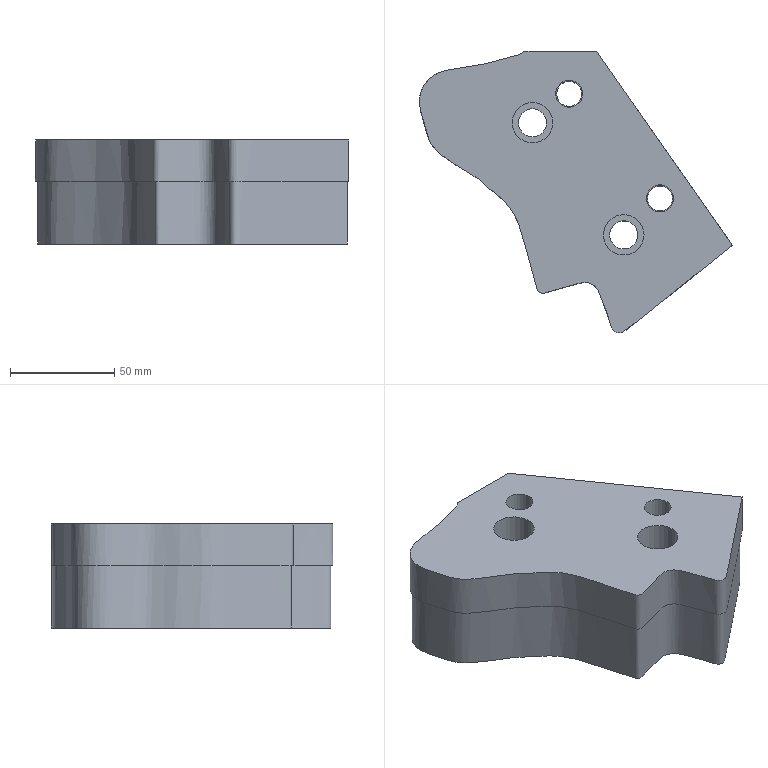Part | NX | features solid 2 | 1 solid | 19 faces | box 150.505 x 135.487 x 50 mm | volume 528166 mm3 | plane 9 | cylinder 8 | spline 2 | commonest cylinder face diameters 12 x2 13 x2 13.5 x2 19.5 x2